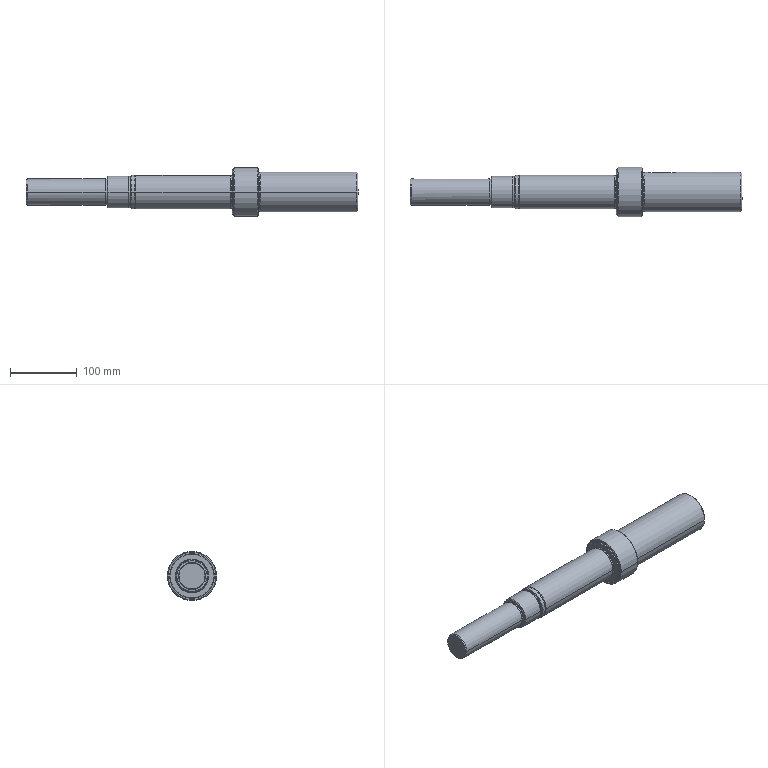Part | SolidWorks | features BaseBody 1 | 1 solid | 88 faces | box 498.34 x 74 x 74 mm | volume 1078927 mm3 | cylinder 30 | cone 26 | spline 17 | plane 15 | commonest cylinder face diameters 50 x4 12 x2 17.294 x2 18 x2 39.5 x2 40 x2